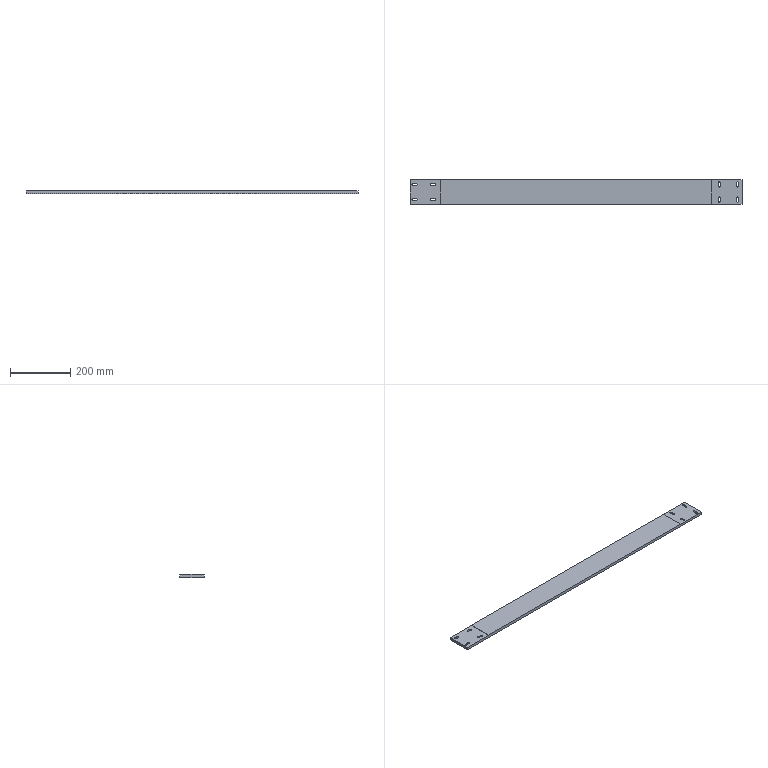Part | SolidWorks | features ICE 2, Extrusion 1, HoleWzd 1 | 1 solid | 46 faces | box 1100 x 80 x 10 mm | volume 856189 mm3 | plane 26 | cylinder 20 | commonest cylinder face diameters 7 x20
STEP:
#1=CARTESIAN_POINT('',(-540.,28.5,9.));
#2=VERTEX_POINT('',#1);
#3=CARTESIAN_POINT('',(-543.5,25.,9.));
#4=VERTEX_POINT('',#3);
#5=CARTESIAN_POINT('',(-540.,25.,9.));
#6=DIRECTION('',(0.,0.,1.));
#7=DIRECTION('',(1.,0.,0.));
#8=AXIS2_PLACEMENT_3D('',#5,#6,#7);
#9=CIRCLE('',#8,3.5);
#10=EDGE_CURVE('',#2,#4,#9,.T.);
#11=ORIENTED_EDGE('',*,*,#10,.T.);
#12=CARTESIAN_POINT('',(-543.5,25.,0.));
#13=VERTEX_POINT('',#12);
#14=CARTESIAN_POINT('',(-543.5,25.,10.));
#15=DIRECTION('',(0.,0.,-1.));
#16=VECTOR('',#15,1000.);
#17=LINE('',#14,#16);
#18=EDGE_CURVE('',#4,#13,#17,.T.);
#19=ORIENTED_EDGE('',*,*,#18,.T.);
#20=CARTESIAN_POINT('',(-540.,28.5,0.));
#21=VERTEX_POINT('',#20);
#22=CARTESIAN_POINT('',(-540.,25.,0.));
#23=DIRECTION('',(0.,0.,-1.));
#24=DIRECTION('',(-1.,0.,0.));
#25=AXIS2_PLACEMENT_3D('',#22,#23,#24);
#26=CIRCLE('',#25,3.5);
#27=EDGE_CURVE('',#13,#21,#26,.T.);
#28=ORIENTED_EDGE('',*,*,#27,.T.);
#29=CARTESIAN_POINT('',(-540.,28.5,10.));
#30=DIRECTION('',(0.,0.,-1.));
#31=VECTOR('',#30,1000.);
#32=LINE('',#29,#31);
#33=EDGE_CURVE('',#2,#21,#32,.T.);
#34=ORIENTED_EDGE('',*,*,#33,.F.);
#35=EDGE_LOOP('',(#11,#19,#28,#34));
#36=FACE_OUTER_BOUND('',#35,.T.);
#37=CARTESIAN_POINT('',(-540.,25.,10.));
#38=DIRECTION('',(0.,0.,-1.));
#39=DIRECTION('',(-1.,0.,0.));
#40=AXIS2_PLACEMENT_3D('',#37,#38,#39);
#41=CYLINDRICAL_SURFACE('',#40,3.5);
#42=ADVANCED_FACE('',(#36),#41,.F.);
#43=CARTESIAN_POINT('',(-540.,-21.5,9.));
#44=VERTEX_POINT('',#43);
#45=CARTESIAN_POINT('',(-543.5,-25.,9.));
#46=VERTEX_POINT('',#45);
#47=CARTESIAN_POINT('',(-540.,-25.,9.));
#48=DIRECTION('',(0.,0.,1.));
#49=DIRECTION('',(1.,0.,0.));
#50=AXIS2_PLACEMENT_3D('',#47,#48,#49);
#51=CIRCLE('',#50,3.5);
#52=EDGE_CURVE('',#44,#46,#51,.T.);
#53=ORIENTED_EDGE('',*,*,#52,.T.);
#54=CARTESIAN_POINT('',(-543.5,-25.,0.));
#55=VERTEX_POINT('',#54);
#56=CARTESIAN_POINT('',(-543.5,-25.,10.));
#57=DIRECTION('',(0.,0.,-1.));
#58=VECTOR('',#57,1000.);
#59=LINE('',#56,#58);
#60=EDGE_CURVE('',#46,#55,#59,.T.);
#61=ORIENTED_EDGE('',*,*,#60,.T.);
#62=CARTESIAN_POINT('',(-540.,-21.5,0.));
#63=VERTEX_POINT('',#62);
#64=CARTESIAN_POINT('',(-540.,-25.,0.));
#65=DIRECTION('',(0.,0.,-1.));
#66=DIRECTION('',(-1.,0.,0.));
#67=AXIS2_PLACEMENT_3D('',#64,#65,#66);
#68=CIRCLE('',#67,3.5);
#69=EDGE_CURVE('',#55,#63,#68,.T.);
#70=ORIENTED_EDGE('',*,*,#69,.T.);
#71=CARTESIAN_POINT('',(-540.,-21.5,10.));
#72=DIRECTION('',(0.,0.,-1.));
#73=VECTOR('',#72,1000.);
#74=LINE('',#71,#73);
#75=EDGE_CURVE('',#44,#63,#74,.T.);
#76=ORIENTED_EDGE('',*,*,#75,.F.);
#77=EDGE_LOOP('',(#53,#61,#70,#76));
#78=FACE_OUTER_BOUND('',#77,.T.);
#79=CARTESIAN_POINT('',(-540.,-25.,10.));
#80=DIRECTION('',(0.,0.,-1.));
#81=DIRECTION('',(-1.,0.,0.));
#82=AXIS2_PLACEMENT_3D('',#79,#80,#81);
#83=CYLINDRICAL_SURFACE('',#82,3.5);
#84=ADVANCED_FACE('',(#78),#83,.F.);
#85=CARTESIAN_POINT('',(-480.,-21.5,9.));
#86=VERTEX_POINT('',#85);
#87=CARTESIAN_POINT('',(-483.5,-25.,9.));
#88=VERTEX_POINT('',#87);
#89=CARTESIAN_POINT('',(-480.,-25.,9.));
#90=DIRECTION('',(0.,0.,1.));
#91=DIRECTION('',(1.,0.,0.));
#92=AXIS2_PLACEMENT_3D('',#89,#90,#91);
#93=CIRCLE('',#92,3.5);
#94=EDGE_CURVE('',#86,#88,#93,.T.);
#95=ORIENTED_EDGE('',*,*,#94,.T.);
#96=CARTESIAN_POINT('',(-483.5,-25.,0.));
#97=VERTEX_POINT('',#96);
#98=CARTESIAN_POINT('',(-483.5,-25.,10.));
#99=DIRECTION('',(0.,0.,-1.));
#100=VECTOR('',#99,1000.);
#101=LINE('',#98,#100);
#102=EDGE_CURVE('',#88,#97,#101,.T.);
#103=ORIENTED_EDGE('',*,*,#102,.T.);
#104=CARTESIAN_POINT('',(-480.,-21.5,0.));
#105=VERTEX_POINT('',#104);
#106=CARTESIAN_POINT('',(-480.,-25.,0.));
#107=DIRECTION('',(0.,0.,-1.));
#108=DIRECTION('',(-1.,0.,0.));
#109=AXIS2_PLACEMENT_3D('',#106,#107,#108);
#110=CIRCLE('',#109,3.5);
#111=EDGE_CURVE('',#97,#105,#110,.T.);
#112=ORIENTED_EDGE('',*,*,#111,.T.);
#113=CARTESIAN_POINT('',(-480.,-21.5,10.));
#114=DIRECTION('',(0.,0.,-1.));
#115=VECTOR('',#114,1000.);
#116=LINE('',#113,#115);
#117=EDGE_CURVE('',#86,#105,#116,.T.);
#118=ORIENTED_EDGE('',*,*,#117,.F.);
#119=EDGE_LOOP('',(#95,#103,#112,#118));
#120=FACE_OUTER_BOUND('',#119,.T.);
#121=CARTESIAN_POINT('',(-480.,-25.,10.));
#122=DIRECTION('',(0.,0.,-1.));
#123=DIRECTION('',(-1.,0.,0.));
#124=AXIS2_PLACEMENT_3D('',#121,#122,#123);
#125=CYLINDRICAL_SURFACE('',#124,3.5);
#126=ADVANCED_FACE('',(#120),#125,.F.);
#127=CARTESIAN_POINT('',(-480.,28.5,9.));
#128=VERTEX_POINT('',#127);
#129=CARTESIAN_POINT('',(-483.5,25.,9.));
#130=VERTEX_POINT('',#129);
#131=CARTESIAN_POINT('',(-480.,25.,9.));
#132=DIRECTION('',(0.,0.,1.));
#133=DIRECTION('',(1.,0.,0.));
#134=AXIS2_PLACEMENT_3D('',#131,#132,#133);
#135=CIRCLE('',#134,3.5);
#136=EDGE_CURVE('',#128,#130,#135,.T.);
#137=ORIENTED_EDGE('',*,*,#136,.T.);
#138=CARTESIAN_POINT('',(-483.5,25.,0.));
#139=VERTEX_POINT('',#138);
#140=CARTESIAN_POINT('',(-483.5,25.,10.));
#141=DIRECTION('',(0.,0.,-1.));
#142=VECTOR('',#141,1000.);
#143=LINE('',#140,#142);
#144=EDGE_CURVE('',#130,#139,#143,.T.);
#145=ORIENTED_EDGE('',*,*,#144,.T.);
#146=CARTESIAN_POINT('',(-480.,28.5,0.));
#147=VERTEX_POINT('',#146);
#148=CARTESIAN_POINT('',(-480.,25.,0.));
#149=DIRECTION('',(0.,0.,-1.));
#150=DIRECTION('',(-1.,0.,0.));
#151=AXIS2_PLACEMENT_3D('',#148,#149,#150);
#152=CIRCLE('',#151,3.5);
#153=EDGE_CURVE('',#139,#147,#152,.T.);
#154=ORIENTED_EDGE('',*,*,#153,.T.);
#155=CARTESIAN_POINT('',(-480.,28.5,10.));
#156=DIRECTION('',(0.,0.,-1.));
#157=VECTOR('',#156,1000.);
#158=LINE('',#155,#157);
#159=EDGE_CURVE('',#128,#147,#158,.T.);
#160=ORIENTED_EDGE('',*,*,#159,.F.);
#161=EDGE_LOOP('',(#137,#145,#154,#160));
#162=FACE_OUTER_BOUND('',#161,.T.);
#163=CARTESIAN_POINT('',(-480.,25.,10.));
#164=DIRECTION('',(0.,0.,-1.));
#165=DIRECTION('',(-1.,0.,0.));
#166=AXIS2_PLACEMENT_3D('',#163,#164,#165);
#167=CYLINDRICAL_SURFACE('',#166,3.5);
#168=ADVANCED_FACE('',(#162),#167,.F.);
#169=CARTESIAN_POINT('',(550.,-40.,9.));
#170=VERTEX_POINT('',#169);
#171=CARTESIAN_POINT('',(550.,40.,9.));
#172=VERTEX_POINT('',#171);
#173=CARTESIAN_POINT('',(550.,40.,9.));
#174=DIRECTION('',(0.,1.,0.));
#175=VECTOR('',#174,1000.);
#176=LINE('',#173,#175);
#177=EDGE_CURVE('',#170,#172,#176,.T.);
#178=ORIENTED_EDGE('',*,*,#177,.F.);
#179=CARTESIAN_POINT('',(550.,-40.,0.));
#180=VERTEX_POINT('',#179);
#181=CARTESIAN_POINT('',(550.,-40.,10.));
#182=DIRECTION('',(0.,0.,-1.));
#183=VECTOR('',#182,1000.);
#184=LINE('',#181,#183);
#185=EDGE_CURVE('',#170,#180,#184,.T.);
#186=ORIENTED_EDGE('',*,*,#185,.T.);
#187=CARTESIAN_POINT('',(550.,40.,0.));
#188=VERTEX_POINT('',#187);
#189=CARTESIAN_POINT('',(550.,40.,0.));
#190=DIRECTION('',(0.,1.,0.));
#191=VECTOR('',#190,1000.);
#192=LINE('',#189,#191);
#193=EDGE_CURVE('',#180,#188,#192,.T.);
#194=ORIENTED_EDGE('',*,*,#193,.T.);
#195=CARTESIAN_POINT('',(550.,40.,10.));
#196=DIRECTION('',(0.,0.,-1.));
#197=VECTOR('',#196,1000.);
#198=LINE('',#195,#197);
#199=EDGE_CURVE('',#172,#188,#198,.T.);
#200=ORIENTED_EDGE('',*,*,#199,.F.);
#201=EDGE_LOOP('',(#178,#186,#194,#200));
#202=FACE_OUTER_BOUND('',#201,.T.);
#203=CARTESIAN_POINT('',(550.,40.,10.));
#204=DIRECTION('',(-1.,0.,0.));
#205=DIRECTION('',(0.,0.,1.));
#206=AXIS2_PLACEMENT_3D('',#203,#204,#205);
#207=PLANE('',#206);
#208=ADVANCED_FACE('',(#202),#207,.F.);
#209=CARTESIAN_POINT('',(-550.,40.,9.));
#210=VERTEX_POINT('',#209);
#211=CARTESIAN_POINT('',(-550.,-40.,9.));
#212=VERTEX_POINT('',#211);
#213=CARTESIAN_POINT('',(-550.,40.,9.));
#214=DIRECTION('',(0.,-1.,0.));
#215=VECTOR('',#214,1000.);
#216=LINE('',#213,#215);
#217=EDGE_CURVE('',#210,#212,#216,.T.);
#218=ORIENTED_EDGE('',*,*,#217,.F.);
#219=CARTESIAN_POINT('',(-550.,40.,0.));
#220=VERTEX_POINT('',#219);
#221=CARTESIAN_POINT('',(-550.,40.,10.));
#222=DIRECTION('',(0.,0.,-1.));
#223=VECTOR('',#222,1000.);
#224=LINE('',#221,#223);
#225=EDGE_CURVE('',#210,#220,#224,.T.);
#226=ORIENTED_EDGE('',*,*,#225,.T.);
#227=CARTESIAN_POINT('',(-550.,-40.,0.));
#228=VERTEX_POINT('',#227);
#229=CARTESIAN_POINT('',(-550.,40.,0.));
#230=DIRECTION('',(0.,-1.,0.));
#231=VECTOR('',#230,1000.);
#232=LINE('',#229,#231);
#233=EDGE_CURVE('',#220,#228,#232,.T.);
#234=ORIENTED_EDGE('',*,*,#233,.T.);
#235=CARTESIAN_POINT('',(-550.,-40.,10.));
#236=DIRECTION('',(0.,0.,-1.));
#237=VECTOR('',#236,1000.);
#238=LINE('',#235,#237);
#239=EDGE_CURVE('',#212,#228,#238,.T.);
#240=ORIENTED_EDGE('',*,*,#239,.F.);
#241=EDGE_LOOP('',(#218,#226,#234,#240));
#242=FACE_OUTER_BOUND('',#241,.T.);
#243=CARTESIAN_POINT('',(-550.,40.,10.));
#244=DIRECTION('',(1.,0.,0.));
#245=DIRECTION('',(0.,0.,-1.));
#246=AXIS2_PLACEMENT_3D('',#243,#244,#245);
#247=PLANE('',#246);
#248=ADVANCED_FACE('',(#242),#247,.F.);
#249=CARTESIAN_POINT('',(-450.,40.,9.));
#250=VERTEX_POINT('',#249);
#251=CARTESIAN_POINT('',(-550.,40.,9.));
#252=DIRECTION('',(-1.,0.,0.));
#253=VECTOR('',#252,1000.);
#254=LINE('',#251,#253);
#255=EDGE_CURVE('',#250,#210,#254,.T.);
#256=ORIENTED_EDGE('',*,*,#255,.F.);
#257=CARTESIAN_POINT('',(-450.,40.,10.));
#258=VERTEX_POINT('',#257);
#259=CARTESIAN_POINT('',(-450.,40.,9.));
#260=DIRECTION('',(0.,0.,1.));
#261=VECTOR('',#260,1000.);
#262=LINE('',#259,#261);
#263=EDGE_CURVE('',#250,#258,#262,.T.);
#264=ORIENTED_EDGE('',*,*,#263,.T.);
#265=CARTESIAN_POINT('',(450.,40.,10.));
#266=VERTEX_POINT('',#265);
#267=CARTESIAN_POINT('',(-550.,40.,10.));
#268=DIRECTION('',(-1.,0.,0.));
#269=VECTOR('',#268,1000.);
#270=LINE('',#267,#269);
#271=EDGE_CURVE('',#266,#258,#270,.T.);
#272=ORIENTED_EDGE('',*,*,#271,.F.);
#273=CARTESIAN_POINT('',(450.,40.,9.));
#274=VERTEX_POINT('',#273);
#275=CARTESIAN_POINT('',(450.,40.,9.));
#276=DIRECTION('',(0.,0.,1.));
#277=VECTOR('',#276,1000.);
#278=LINE('',#275,#277);
#279=EDGE_CURVE('',#274,#266,#278,.T.);
#280=ORIENTED_EDGE('',*,*,#279,.F.);
#281=CARTESIAN_POINT('',(550.,40.,9.));
#282=DIRECTION('',(-1.,0.,0.));
#283=VECTOR('',#282,1000.);
#284=LINE('',#281,#283);
#285=EDGE_CURVE('',#172,#274,#284,.T.);
#286=ORIENTED_EDGE('',*,*,#285,.F.);
#287=ORIENTED_EDGE('',*,*,#199,.T.);
#288=CARTESIAN_POINT('',(-550.,40.,0.));
#289=DIRECTION('',(-1.,0.,0.));
#290=VECTOR('',#289,1000.);
#291=LINE('',#288,#290);
#292=EDGE_CURVE('',#188,#220,#291,.T.);
#293=ORIENTED_EDGE('',*,*,#292,.T.);
#294=ORIENTED_EDGE('',*,*,#225,.F.);
#295=EDGE_LOOP('',(#256,#264,#272,#280,#286,#287,#293,#294));
#296=FACE_OUTER_BOUND('',#295,.T.);
#297=CARTESIAN_POINT('',(-550.,40.,10.));
#298=DIRECTION('',(0.,-1.,0.));
#299=DIRECTION('',(0.,0.,-1.));
#300=AXIS2_PLACEMENT_3D('',#297,#298,#299);
#301=PLANE('',#300);
#302=ADVANCED_FACE('',(#296),#301,.F.);
#303=CARTESIAN_POINT('',(-450.,-40.,10.));
#304=VERTEX_POINT('',#303);
#305=CARTESIAN_POINT('',(450.,-40.,10.));
#306=VERTEX_POINT('',#305);
#307=CARTESIAN_POINT('',(-550.,-40.,10.));
#308=DIRECTION('',(1.,0.,0.));
#309=VECTOR('',#308,1000.);
#310=LINE('',#307,#309);
#311=EDGE_CURVE('',#304,#306,#310,.T.);
#312=ORIENTED_EDGE('',*,*,#311,.F.);
#313=CARTESIAN_POINT('',(-450.,-40.,9.));
#314=VERTEX_POINT('',#313);
#315=CARTESIAN_POINT('',(-450.,-40.,9.));
#316=DIRECTION('',(0.,0.,1.));
#317=VECTOR('',#316,1000.);
#318=LINE('',#315,#317);
#319=EDGE_CURVE('',#314,#304,#318,.T.);
#320=ORIENTED_EDGE('',*,*,#319,.F.);
#321=CARTESIAN_POINT('',(-550.,-40.,9.));
#322=DIRECTION('',(1.,0.,0.));
#323=VECTOR('',#322,1000.);
#324=LINE('',#321,#323);
#325=EDGE_CURVE('',#212,#314,#324,.T.);
#326=ORIENTED_EDGE('',*,*,#325,.F.);
#327=ORIENTED_EDGE('',*,*,#239,.T.);
#328=CARTESIAN_POINT('',(-550.,-40.,0.));
#329=DIRECTION('',(1.,0.,0.));
#330=VECTOR('',#329,1000.);
#331=LINE('',#328,#330);
#332=EDGE_CURVE('',#228,#180,#331,.T.);
#333=ORIENTED_EDGE('',*,*,#332,.T.);
#334=ORIENTED_EDGE('',*,*,#185,.F.);
#335=CARTESIAN_POINT('',(450.,-40.,9.));
#336=VERTEX_POINT('',#335);
#337=CARTESIAN_POINT('',(550.,-40.,9.));
#338=DIRECTION('',(1.,0.,0.));
#339=VECTOR('',#338,1000.);
#340=LINE('',#337,#339);
#341=EDGE_CURVE('',#336,#170,#340,.T.);
#342=ORIENTED_EDGE('',*,*,#341,.F.);
#343=CARTESIAN_POINT('',(450.,-40.,9.));
#344=DIRECTION('',(0.,0.,1.));
#345=VECTOR('',#344,1000.);
#346=LINE('',#343,#345);
#347=EDGE_CURVE('',#336,#306,#346,.T.);
#348=ORIENTED_EDGE('',*,*,#347,.T.);
#349=EDGE_LOOP('',(#312,#320,#326,#327,#333,#334,#342,#348));
#350=FACE_OUTER_BOUND('',#349,.T.);
#351=CARTESIAN_POINT('',(-550.,-40.,10.));
#352=DIRECTION('',(0.,1.,0.));
#353=DIRECTION('',(0.,0.,1.));
#354=AXIS2_PLACEMENT_3D('',#351,#352,#353);
#355=PLANE('',#354);
#356=ADVANCED_FACE('',(#350),#355,.F.);
#357=CARTESIAN_POINT('',(-450.,40.,10.));
#358=DIRECTION('',(0.,1.,0.));
#359=VECTOR('',#358,1000.);
#360=LINE('',#357,#359);
#361=EDGE_CURVE('',#304,#258,#360,.T.);
#362=ORIENTED_EDGE('',*,*,#361,.F.);
#363=ORIENTED_EDGE('',*,*,#311,.T.);
#364=CARTESIAN_POINT('',(450.,40.,10.));
#365=DIRECTION('',(0.,-1.,0.));
#366=VECTOR('',#365,1000.);
#367=LINE('',#364,#366);
#368=EDGE_CURVE('',#266,#306,#367,.T.);
#369=ORIENTED_EDGE('',*,*,#368,.F.);
#370=ORIENTED_EDGE('',*,*,#271,.T.);
#371=EDGE_LOOP('',(#362,#363,#369,#370));
#372=FACE_OUTER_BOUND('',#371,.T.);
#373=CARTESIAN_POINT('',(0.,0.,10.));
#374=DIRECTION('',(0.,0.,1.));
#375=DIRECTION('',(1.,0.,0.));
#376=AXIS2_PLACEMENT_3D('',#373,#374,#375);
#377=PLANE('',#376);
#378=ADVANCED_FACE('',(#372),#377,.T.);
#379=CARTESIAN_POINT('',(-470.,-28.5,0.));
#380=VERTEX_POINT('',#379);
#381=CARTESIAN_POINT('',(-480.,-28.5,0.));
#382=VERTEX_POINT('',#381);
#383=CARTESIAN_POINT('',(-470.,-28.5,0.));
#384=DIRECTION('',(-1.,0.,0.));
#385=VECTOR('',#384,1000.);
#386=LINE('',#383,#385);
#387=EDGE_CURVE('',#380,#382,#386,.T.);
#388=ORIENTED_EDGE('',*,*,#387,.F.);
#389=CARTESIAN_POINT('',(-470.,-21.5,0.));
#390=VERTEX_POINT('',#389);
#391=CARTESIAN_POINT('',(-470.,-25.,0.));
#392=DIRECTION('',(0.,0.,-1.));
#393=DIRECTION('',(-1.,0.,0.));
#394=AXIS2_PLACEMENT_3D('',#391,#392,#393);
#395=CIRCLE('',#394,3.5);
#396=EDGE_CURVE('',#390,#380,#395,.T.);
#397=ORIENTED_EDGE('',*,*,#396,.F.);
#398=CARTESIAN_POINT('',(-470.,-21.5,0.));
#399=DIRECTION('',(1.,0.,0.));
#400=VECTOR('',#399,1000.);
#401=LINE('',#398,#400);
#402=EDGE_CURVE('',#105,#390,#401,.T.);
#403=ORIENTED_EDGE('',*,*,#402,.F.);
#404=ORIENTED_EDGE('',*,*,#111,.F.);
#405=CARTESIAN_POINT('',(-480.,-25.,0.));
#406=DIRECTION('',(0.,0.,-1.));
#407=DIRECTION('',(-1.,0.,0.));
#408=AXIS2_PLACEMENT_3D('',#405,#406,#407);
#409=CIRCLE('',#408,3.5);
#410=EDGE_CURVE('',#382,#97,#409,.T.);
#411=ORIENTED_EDGE('',*,*,#410,.F.);
#412=EDGE_LOOP('',(#388,#397,#403,#404,#411));
#413=FACE_BOUND('',#412,.T.);
#414=CARTESIAN_POINT('',(-530.,21.5,0.));
#415=VERTEX_POINT('',#414);
#416=CARTESIAN_POINT('',(-540.,21.5,0.));
#417=VERTEX_POINT('',#416);
#418=CARTESIAN_POINT('',(-530.,21.5,0.));
#419=DIRECTION('',(-1.,0.,0.));
#420=VECTOR('',#419,1000.);
#421=LINE('',#418,#420);
#422=EDGE_CURVE('',#415,#417,#421,.T.);
#423=ORIENTED_EDGE('',*,*,#422,.F.);
#424=CARTESIAN_POINT('',(-530.,28.5,0.));
#425=VERTEX_POINT('',#424);
#426=CARTESIAN_POINT('',(-530.,25.,0.));
#427=DIRECTION('',(0.,0.,-1.));
#428=DIRECTION('',(-1.,0.,0.));
#429=AXIS2_PLACEMENT_3D('',#426,#427,#428);
#430=CIRCLE('',#429,3.5);
#431=EDGE_CURVE('',#425,#415,#430,.T.);
#432=ORIENTED_EDGE('',*,*,#431,.F.);
#433=CARTESIAN_POINT('',(-530.,28.5,0.));
#434=DIRECTION('',(1.,0.,0.));
#435=VECTOR('',#434,1000.);
#436=LINE('',#433,#435);
#437=EDGE_CURVE('',#21,#425,#436,.T.);
#438=ORIENTED_EDGE('',*,*,#437,.F.);
#439=ORIENTED_EDGE('',*,*,#27,.F.);
#440=CARTESIAN_POINT('',(-540.,25.,0.));
#441=DIRECTION('',(0.,0.,-1.));
#442=DIRECTION('',(-1.,0.,0.));
#443=AXIS2_PLACEMENT_3D('',#440,#441,#442);
#444=CIRCLE('',#443,3.5);
#445=EDGE_CURVE('',#417,#13,#444,.T.);
#446=ORIENTED_EDGE('',*,*,#445,.F.);
#447=EDGE_LOOP('',(#423,#432,#438,#439,#446));
#448=FACE_BOUND('',#447,.T.);
#449=CARTESIAN_POINT('',(-530.,-28.5,0.));
#450=VERTEX_POINT('',#449);
#451=CARTESIAN_POINT('',(-540.,-28.5,0.));
#452=VERTEX_POINT('',#451);
#453=CARTESIAN_POINT('',(-530.,-28.5,0.));
#454=DIRECTION('',(-1.,0.,0.));
#455=VECTOR('',#454,1000.);
#456=LINE('',#453,#455);
#457=EDGE_CURVE('',#450,#452,#456,.T.);
#458=ORIENTED_EDGE('',*,*,#457,.F.);
#459=CARTESIAN_POINT('',(-530.,-21.5,0.));
#460=VERTEX_POINT('',#459);
#461=CARTESIAN_POINT('',(-530.,-25.,0.));
#462=DIRECTION('',(0.,0.,-1.));
#463=DIRECTION('',(-1.,0.,0.));
#464=AXIS2_PLACEMENT_3D('',#461,#462,#463);
#465=CIRCLE('',#464,3.5);
#466=EDGE_CURVE('',#460,#450,#465,.T.);
#467=ORIENTED_EDGE('',*,*,#466,.F.);
#468=CARTESIAN_POINT('',(-530.,-21.5,0.));
#469=DIRECTION('',(1.,0.,0.));
#470=VECTOR('',#469,1000.);
#471=LINE('',#468,#470);
#472=EDGE_CURVE('',#63,#460,#471,.T.);
#473=ORIENTED_EDGE('',*,*,#472,.F.);
#474=ORIENTED_EDGE('',*,*,#69,.F.);
#475=CARTESIAN_POINT('',(-540.,-25.,0.));
#476=DIRECTION('',(0.,0.,-1.));
#477=DIRECTION('',(-1.,0.,0.));
#478=AXIS2_PLACEMENT_3D('',#475,#476,#477);
#479=CIRCLE('',#478,3.5);
#480=EDGE_CURVE('',#452,#55,#479,.T.);
#481=ORIENTED_EDGE('',*,*,#480,.F.);
#482=EDGE_LOOP('',(#458,#467,#473,#474,#481));
#483=FACE_BOUND('',#482,.T.);
#484=CARTESIAN_POINT('',(-470.,21.5,0.));
#485=VERTEX_POINT('',#484);
#486=CARTESIAN_POINT('',(-480.,21.5,0.));
#487=VERTEX_POINT('',#486);
#488=CARTESIAN_POINT('',(-470.,21.5,0.));
#489=DIRECTION('',(-1.,0.,0.));
#490=VECTOR('',#489,1000.);
#491=LINE('',#488,#490);
#492=EDGE_CURVE('',#485,#487,#491,.T.);
#493=ORIENTED_EDGE('',*,*,#492,.F.);
#494=CARTESIAN_POINT('',(-470.,28.5,0.));
#495=VERTEX_POINT('',#494);
#496=CARTESIAN_POINT('',(-470.,25.,0.));
#497=DIRECTION('',(0.,0.,-1.));
#498=DIRECTION('',(-1.,0.,0.));
#499=AXIS2_PLACEMENT_3D('',#496,#497,#498);
#500=CIRCLE('',#499,3.5);
#501=EDGE_CURVE('',#495,#485,#500,.T.);
#502=ORIENTED_EDGE('',*,*,#501,.F.);
#503=CARTESIAN_POINT('',(-470.,28.5,0.));
#504=DIRECTION('',(1.,0.,0.));
#505=VECTOR('',#504,1000.);
#506=LINE('',#503,#505);
#507=EDGE_CURVE('',#147,#495,#506,.T.);
#508=ORIENTED_EDGE('',*,*,#507,.F.);
#509=ORIENTED_EDGE('',*,*,#153,.F.);
#510=CARTESIAN_POINT('',(-480.,25.,0.));
#511=DIRECTION('',(0.,0.,-1.));
#512=DIRECTION('',(-1.,0.,0.));
#513=AXIS2_PLACEMENT_3D('',#510,#511,#512);
#514=CIRCLE('',#513,3.5);
#515=EDGE_CURVE('',#487,#139,#514,.T.);
#516=ORIENTED_EDGE('',*,*,#515,.F.);
#517=EDGE_LOOP('',(#493,#502,#508,#509,#516));
#518=FACE_BOUND('',#517,.T.);
#519=CARTESIAN_POINT('',(478.5,30.,0.));
#520=VERTEX_POINT('',#519);
#521=CARTESIAN_POINT('',(478.5,20.,0.));
#522=VERTEX_POINT('',#521);
#523=CARTESIAN_POINT('',(478.5,30.,0.));
#524=DIRECTION('',(0.,-1.,0.));
#525=VECTOR('',#524,1000.);
#526=LINE('',#523,#525);
#527=EDGE_CURVE('',#520,#522,#526,.T.);
#528=ORIENTED_EDGE('',*,*,#527,.F.);
#529=CARTESIAN_POINT('',(471.5,30.,0.));
#530=VERTEX_POINT('',#529);
#531=CARTESIAN_POINT('',(475.,30.,0.));
#532=DIRECTION('',(0.,0.,-1.));
#533=DIRECTION('',(-1.,0.,0.));
#534=AXIS2_PLACEMENT_3D('',#531,#532,#533);
#535=CIRCLE('',#534,3.5);
#536=EDGE_CURVE('',#530,#520,#535,.T.);
#537=ORIENTED_EDGE('',*,*,#536,.F.);
#538=CARTESIAN_POINT('',(471.5,20.,0.));
#539=VERTEX_POINT('',#538);
#540=CARTESIAN_POINT('',(471.5,30.,0.));
#541=DIRECTION('',(0.,1.,0.));
#542=VECTOR('',#541,1000.);
#543=LINE('',#540,#542);
#544=EDGE_CURVE('',#539,#530,#543,.T.);
#545=ORIENTED_EDGE('',*,*,#544,.F.);
#546=CARTESIAN_POINT('',(475.,20.,0.));
#547=DIRECTION('',(0.,0.,-1.));
#548=DIRECTION('',(-1.,0.,0.));
#549=AXIS2_PLACEMENT_3D('',#546,#547,#548);
#550=CIRCLE('',#549,3.5);
#551=EDGE_CURVE('',#522,#539,#550,.T.);
#552=ORIENTED_EDGE('',*,*,#551,.F.);
#553=EDGE_LOOP('',(#528,#537,#545,#552));
#554=FACE_BOUND('',#553,.T.);
#555=CARTESIAN_POINT('',(471.5,-30.,0.));
#556=VERTEX_POINT('',#555);
#557=CARTESIAN_POINT('',(471.5,-20.,0.));
#558=VERTEX_POINT('',#557);
#559=CARTESIAN_POINT('',(471.5,-30.,0.));
#560=DIRECTION('',(0.,1.,0.));
#561=VECTOR('',#560,1000.);
#562=LINE('',#559,#561);
#563=EDGE_CURVE('',#556,#558,#562,.T.);
#564=ORIENTED_EDGE('',*,*,#563,.F.);
#565=CARTESIAN_POINT('',(478.5,-30.,0.));
#566=VERTEX_POINT('',#565);
#567=CARTESIAN_POINT('',(475.,-30.,0.));
#568=DIRECTION('',(0.,0.,-1.));
#569=DIRECTION('',(-1.,0.,0.));
#570=AXIS2_PLACEMENT_3D('',#567,#568,#569);
#571=CIRCLE('',#570,3.5);
#572=EDGE_CURVE('',#566,#556,#571,.T.);
#573=ORIENTED_EDGE('',*,*,#572,.F.);
#574=CARTESIAN_POINT('',(478.5,-20.,0.));
#575=VERTEX_POINT('',#574);
#576=CARTESIAN_POINT('',(478.5,-30.,0.));
#577=DIRECTION('',(0.,-1.,0.));
#578=VECTOR('',#577,1000.);
#579=LINE('',#576,#578);
#580=EDGE_CURVE('',#575,#566,#579,.T.);
#581=ORIENTED_EDGE('',*,*,#580,.F.);
#582=CARTESIAN_POINT('',(475.,-20.,0.));
#583=DIRECTION('',(0.,0.,-1.));
#584=DIRECTION('',(-1.,0.,0.));
#585=AXIS2_PLACEMENT_3D('',#582,#583,#584);
#586=CIRCLE('',#585,3.5);
#587=EDGE_CURVE('',#558,#575,#586,.T.);
#588=ORIENTED_EDGE('',*,*,#587,.F.);
#589=EDGE_LOOP('',(#564,#573,#581,#588));
#590=FACE_BOUND('',#589,.T.);
#591=CARTESIAN_POINT('',(531.5,-30.,0.));
#592=VERTEX_POINT('',#591);
#593=CARTESIAN_POINT('',(531.5,-20.,0.));
#594=VERTEX_POINT('',#593);
#595=CARTESIAN_POINT('',(531.5,-30.,0.));
#596=DIRECTION('',(0.,1.,0.));
#597=VECTOR('',#596,1000.);
#598=LINE('',#595,#597);
#599=EDGE_CURVE('',#592,#594,#598,.T.);
#600=ORIENTED_EDGE('',*,*,#599,.F.);
#601=CARTESIAN_POINT('',(538.5,-30.,0.));
#602=VERTEX_POINT('',#601);
#603=CARTESIAN_POINT('',(535.,-30.,0.));
#604=DIRECTION('',(0.,0.,-1.));
#605=DIRECTION('',(-1.,0.,0.));
#606=AXIS2_PLACEMENT_3D('',#603,#604,#605);
#607=CIRCLE('',#606,3.5);
#608=EDGE_CURVE('',#602,#592,#607,.T.);
#609=ORIENTED_EDGE('',*,*,#608,.F.);
#610=CARTESIAN_POINT('',(538.5,-20.,0.));
#611=VERTEX_POINT('',#610);
#612=CARTESIAN_POINT('',(538.5,-30.,0.));
#613=DIRECTION('',(0.,-1.,0.));
#614=VECTOR('',#613,1000.);
#615=LINE('',#612,#614);
#616=EDGE_CURVE('',#611,#602,#615,.T.);
#617=ORIENTED_EDGE('',*,*,#616,.F.);
#618=CARTESIAN_POINT('',(535.,-20.,0.));
#619=DIRECTION('',(0.,0.,-1.));
#620=DIRECTION('',(-1.,0.,0.));
#621=AXIS2_PLACEMENT_3D('',#618,#619,#620);
#622=CIRCLE('',#621,3.5);
#623=EDGE_CURVE('',#594,#611,#622,.T.);
#624=ORIENTED_EDGE('',*,*,#623,.F.);
#625=EDGE_LOOP('',(#600,#609,#617,#624));
#626=FACE_BOUND('',#625,.T.);
#627=CARTESIAN_POINT('',(538.5,30.,0.));
#628=VERTEX_POINT('',#627);
#629=CARTESIAN_POINT('',(538.5,20.,0.));
#630=VERTEX_POINT('',#629);
#631=CARTESIAN_POINT('',(538.5,30.,0.));
#632=DIRECTION('',(0.,-1.,0.));
#633=VECTOR('',#632,1000.);
#634=LINE('',#631,#633);
#635=EDGE_CURVE('',#628,#630,#634,.T.);
#636=ORIENTED_EDGE('',*,*,#635,.F.);
#637=CARTESIAN_POINT('',(531.5,30.,0.));
#638=VERTEX_POINT('',#637);
#639=CARTESIAN_POINT('',(535.,30.,0.));
#640=DIRECTION('',(0.,0.,-1.));
#641=DIRECTION('',(-1.,0.,0.));
#642=AXIS2_PLACEMENT_3D('',#639,#640,#641);
#643=CIRCLE('',#642,3.5);
#644=EDGE_CURVE('',#638,#628,#643,.T.);
#645=ORIENTED_EDGE('',*,*,#644,.F.);
#646=CARTESIAN_POINT('',(531.5,20.,0.));
#647=VERTEX_POINT('',#646);
#648=CARTESIAN_POINT('',(531.5,30.,0.));
#649=DIRECTION('',(0.,1.,0.));
#650=VECTOR('',#649,1000.);
#651=LINE('',#648,#650);
#652=EDGE_CURVE('',#647,#638,#651,.T.);
#653=ORIENTED_EDGE('',*,*,#652,.F.);
#654=CARTESIAN_POINT('',(535.,20.,0.));
#655=DIRECTION('',(0.,0.,-1.));
#656=DIRECTION('',(-1.,0.,0.));
#657=AXIS2_PLACEMENT_3D('',#654,#655,#656);
#658=CIRCLE('',#657,3.5);
#659=EDGE_CURVE('',#630,#647,#658,.T.);
#660=ORIENTED_EDGE('',*,*,#659,.F.);
#661=EDGE_LOOP('',(#636,#645,#653,#660));
#662=FACE_BOUND('',#661,.T.);
#663=ORIENTED_EDGE('',*,*,#193,.F.);
#664=ORIENTED_EDGE('',*,*,#332,.F.);
#665=ORIENTED_EDGE('',*,*,#233,.F.);
#666=ORIENTED_EDGE('',*,*,#292,.F.);
#667=EDGE_LOOP('',(#663,#664,#665,#666));
#668=FACE_OUTER_BOUND('',#667,.T.);
#669=CARTESIAN_POINT('',(0.,0.,0.));
#670=DIRECTION('',(0.,0.,1.));
#671=DIRECTION('',(1.,0.,0.));
#672=AXIS2_PLACEMENT_3D('',#669,#670,#671);
#673=PLANE('',#672);
#674=ADVANCED_FACE('',(#413,#448,#483,#518,#554,#590,#626,#662,#668),#673,.F.);
#675=ORIENTED_EDGE('',*,*,#368,.T.);
#676=ORIENTED_EDGE('',*,*,#347,.F.);
#677=CARTESIAN_POINT('',(450.,40.,9.));
#678=DIRECTION('',(0.,-1.,0.));
#679=VECTOR('',#678,1000.);
#680=LINE('',#677,#679);
#681=EDGE_CURVE('',#274,#336,#680,.T.);
#682=ORIENTED_EDGE('',*,*,#681,.F.);
#683=ORIENTED_EDGE('',*,*,#279,.T.);
#684=EDGE_LOOP('',(#675,#676,#682,#683));
#685=FACE_OUTER_BOUND('',#684,.T.);
#686=CARTESIAN_POINT('',(450.,40.,9.));
#687=DIRECTION('',(-1.,0.,0.));
#688=DIRECTION('',(0.,0.,1.));
#689=AXIS2_PLACEMENT_3D('',#686,#687,#688);
#690=PLANE('',#689);
#691=ADVANCED_FACE('',(#685),#690,.F.);
#692=CARTESIAN_POINT('',(538.5,30.,9.));
#693=VERTEX_POINT('',#692);
#694=CARTESIAN_POINT('',(531.5,30.,9.));
#695=VERTEX_POINT('',#694);
#696=CARTESIAN_POINT('',(535.,30.,9.));
#697=DIRECTION('',(0.,0.,1.));
#698=DIRECTION('',(1.,0.,0.));
#699=AXIS2_PLACEMENT_3D('',#696,#697,#698);
#700=CIRCLE('',#699,3.5);
#701=EDGE_CURVE('',#693,#695,#700,.T.);
#702=ORIENTED_EDGE('',*,*,#701,.F.);
#703=CARTESIAN_POINT('',(538.5,20.,9.));
#704=VERTEX_POINT('',#703);
#705=CARTESIAN_POINT('',(538.5,0.,9.));
#706=DIRECTION('',(0.,1.,0.));
#707=VECTOR('',#706,1000.);
#708=LINE('',#705,#707);
#709=EDGE_CURVE('',#704,#693,#708,.T.);
#710=ORIENTED_EDGE('',*,*,#709,.F.);
#711=CARTESIAN_POINT('',(531.5,20.,9.));
#712=VERTEX_POINT('',#711);
#713=CARTESIAN_POINT('',(535.,20.,9.));
#714=DIRECTION('',(0.,0.,1.));
#715=DIRECTION('',(1.,0.,0.));
#716=AXIS2_PLACEMENT_3D('',#713,#714,#715);
#717=CIRCLE('',#716,3.5);
#718=EDGE_CURVE('',#712,#704,#717,.T.);
#719=ORIENTED_EDGE('',*,*,#718,.F.);
#720=CARTESIAN_POINT('',(531.5,0.,9.));
#721=DIRECTION('',(0.,-1.,0.));
#722=VECTOR('',#721,1000.);
#723=LINE('',#720,#722);
#724=EDGE_CURVE('',#695,#712,#723,.T.);
#725=ORIENTED_EDGE('',*,*,#724,.F.);
#726=EDGE_LOOP('',(#702,#710,#719,#725));
#727=FACE_BOUND('',#726,.T.);
#728=CARTESIAN_POINT('',(471.5,-30.,9.));
#729=VERTEX_POINT('',#728);
#730=CARTESIAN_POINT('',(478.5,-30.,9.));
#731=VERTEX_POINT('',#730);
#732=CARTESIAN_POINT('',(475.,-30.,9.));
#733=DIRECTION('',(0.,0.,1.));
#734=DIRECTION('',(1.,0.,0.));
#735=AXIS2_PLACEMENT_3D('',#732,#733,#734);
#736=CIRCLE('',#735,3.5);
#737=EDGE_CURVE('',#729,#731,#736,.T.);
#738=ORIENTED_EDGE('',*,*,#737,.F.);
#739=CARTESIAN_POINT('',(471.5,-20.,9.));
#740=VERTEX_POINT('',#739);
#741=CARTESIAN_POINT('',(471.5,0.,9.));
#742=DIRECTION('',(0.,-1.,0.));
#743=VECTOR('',#742,1000.);
#744=LINE('',#741,#743);
#745=EDGE_CURVE('',#740,#729,#744,.T.);
#746=ORIENTED_EDGE('',*,*,#745,.F.);
#747=CARTESIAN_POINT('',(478.5,-20.,9.));
#748=VERTEX_POINT('',#747);
#749=CARTESIAN_POINT('',(475.,-20.,9.));
#750=DIRECTION('',(0.,0.,1.));
#751=DIRECTION('',(1.,0.,0.));
#752=AXIS2_PLACEMENT_3D('',#749,#750,#751);
#753=CIRCLE('',#752,3.5);
#754=EDGE_CURVE('',#748,#740,#753,.T.);
#755=ORIENTED_EDGE('',*,*,#754,.F.);
#756=CARTESIAN_POINT('',(478.5,0.,9.));
#757=DIRECTION('',(0.,1.,0.));
#758=VECTOR('',#757,1000.);
#759=LINE('',#756,#758);
#760=EDGE_CURVE('',#731,#748,#759,.T.);
#761=ORIENTED_EDGE('',*,*,#760,.F.);
#762=EDGE_LOOP('',(#738,#746,#755,#761));
#763=FACE_BOUND('',#762,.T.);
#764=CARTESIAN_POINT('',(531.5,-30.,9.));
#765=VERTEX_POINT('',#764);
#766=CARTESIAN_POINT('',(538.5,-30.,9.));
#767=VERTEX_POINT('',#766);
#768=CARTESIAN_POINT('',(535.,-30.,9.));
#769=DIRECTION('',(0.,0.,1.));
#770=DIRECTION('',(1.,0.,0.));
#771=AXIS2_PLACEMENT_3D('',#768,#769,#770);
#772=CIRCLE('',#771,3.5);
#773=EDGE_CURVE('',#765,#767,#772,.T.);
#774=ORIENTED_EDGE('',*,*,#773,.F.);
#775=CARTESIAN_POINT('',(531.5,-20.,9.));
#776=VERTEX_POINT('',#775);
#777=CARTESIAN_POINT('',(531.5,0.,9.));
#778=DIRECTION('',(0.,-1.,0.));
#779=VECTOR('',#778,1000.);
#780=LINE('',#777,#779);
#781=EDGE_CURVE('',#776,#765,#780,.T.);
#782=ORIENTED_EDGE('',*,*,#781,.F.);
#783=CARTESIAN_POINT('',(538.5,-20.,9.));
#784=VERTEX_POINT('',#783);
#785=CARTESIAN_POINT('',(535.,-20.,9.));
#786=DIRECTION('',(0.,0.,1.));
#787=DIRECTION('',(1.,0.,0.));
#788=AXIS2_PLACEMENT_3D('',#785,#786,#787);
#789=CIRCLE('',#788,3.5);
#790=EDGE_CURVE('',#784,#776,#789,.T.);
#791=ORIENTED_EDGE('',*,*,#790,.F.);
#792=CARTESIAN_POINT('',(538.5,0.,9.));
#793=DIRECTION('',(0.,1.,0.));
#794=VECTOR('',#793,1000.);
#795=LINE('',#792,#794);
#796=EDGE_CURVE('',#767,#784,#795,.T.);
#797=ORIENTED_EDGE('',*,*,#796,.F.);
#798=EDGE_LOOP('',(#774,#782,#791,#797));
#799=FACE_BOUND('',#798,.T.);
#800=CARTESIAN_POINT('',(478.5,30.,9.));
#801=VERTEX_POINT('',#800);
#802=CARTESIAN_POINT('',(471.5,30.,9.));
#803=VERTEX_POINT('',#802);
#804=CARTESIAN_POINT('',(475.,30.,9.));
#805=DIRECTION('',(0.,0.,1.));
#806=DIRECTION('',(1.,0.,0.));
#807=AXIS2_PLACEMENT_3D('',#804,#805,#806);
#808=CIRCLE('',#807,3.5);
#809=EDGE_CURVE('',#801,#803,#808,.T.);
#810=ORIENTED_EDGE('',*,*,#809,.F.);
#811=CARTESIAN_POINT('',(478.5,20.,9.));
#812=VERTEX_POINT('',#811);
#813=CARTESIAN_POINT('',(478.5,0.,9.));
#814=DIRECTION('',(0.,1.,0.));
#815=VECTOR('',#814,1000.);
#816=LINE('',#813,#815);
#817=EDGE_CURVE('',#812,#801,#816,.T.);
#818=ORIENTED_EDGE('',*,*,#817,.F.);
#819=CARTESIAN_POINT('',(471.5,20.,9.));
#820=VERTEX_POINT('',#819);
#821=CARTESIAN_POINT('',(475.,20.,9.));
#822=DIRECTION('',(0.,0.,1.));
#823=DIRECTION('',(1.,0.,0.));
#824=AXIS2_PLACEMENT_3D('',#821,#822,#823);
#825=CIRCLE('',#824,3.5);
#826=EDGE_CURVE('',#820,#812,#825,.T.);
#827=ORIENTED_EDGE('',*,*,#826,.F.);
#828=CARTESIAN_POINT('',(471.5,0.,9.));
#829=DIRECTION('',(0.,-1.,0.));
#830=VECTOR('',#829,1000.);
#831=LINE('',#828,#830);
#832=EDGE_CURVE('',#803,#820,#831,.T.);
#833=ORIENTED_EDGE('',*,*,#832,.F.);
#834=EDGE_LOOP('',(#810,#818,#827,#833));
#835=FACE_BOUND('',#834,.T.);
#836=ORIENTED_EDGE('',*,*,#285,.T.);
#837=ORIENTED_EDGE('',*,*,#681,.T.);
#838=ORIENTED_EDGE('',*,*,#341,.T.);
#839=ORIENTED_EDGE('',*,*,#177,.T.);
#840=EDGE_LOOP('',(#836,#837,#838,#839));
#841=FACE_OUTER_BOUND('',#840,.T.);
#842=CARTESIAN_POINT('',(0.,0.,9.));
#843=DIRECTION('',(0.,0.,1.));
#844=DIRECTION('',(1.,0.,0.));
#845=AXIS2_PLACEMENT_3D('',#842,#843,#844);
#846=PLANE('',#845);
#847=ADVANCED_FACE('',(#727,#763,#799,#835,#841),#846,.T.);
#848=ORIENTED_EDGE('',*,*,#361,.T.);
#849=ORIENTED_EDGE('',*,*,#263,.F.);
#850=CARTESIAN_POINT('',(-450.,40.,9.));
#851=DIRECTION('',(0.,1.,0.));
#852=VECTOR('',#851,1000.);
#853=LINE('',#850,#852);
#854=EDGE_CURVE('',#314,#250,#853,.T.);
#855=ORIENTED_EDGE('',*,*,#854,.F.);
#856=ORIENTED_EDGE('',*,*,#319,.T.);
#857=EDGE_LOOP('',(#848,#849,#855,#856));
#858=FACE_OUTER_BOUND('',#857,.T.);
#859=CARTESIAN_POINT('',(-450.,40.,9.));
#860=DIRECTION('',(1.,0.,0.));
#861=DIRECTION('',(0.,0.,-1.));
#862=AXIS2_PLACEMENT_3D('',#859,#860,#861);
#863=PLANE('',#862);
#864=ADVANCED_FACE('',(#858),#863,.F.);
#865=CARTESIAN_POINT('',(-530.,21.5,9.));
#866=VERTEX_POINT('',#865);
#867=CARTESIAN_POINT('',(-530.,28.5,9.));
#868=VERTEX_POINT('',#867);
#869=CARTESIAN_POINT('',(-530.,25.,9.));
#870=DIRECTION('',(0.,0.,1.));
#871=DIRECTION('',(1.,0.,0.));
#872=AXIS2_PLACEMENT_3D('',#869,#870,#871);
#873=CIRCLE('',#872,3.5);
#874=EDGE_CURVE('',#866,#868,#873,.T.);
#875=ORIENTED_EDGE('',*,*,#874,.F.);
#876=CARTESIAN_POINT('',(-540.,21.5,9.));
#877=VERTEX_POINT('',#876);
#878=CARTESIAN_POINT('',(0.,21.5,9.));
#879=DIRECTION('',(1.,0.,0.));
#880=VECTOR('',#879,1000.);
#881=LINE('',#878,#880);
#882=EDGE_CURVE('',#877,#866,#881,.T.);
#883=ORIENTED_EDGE('',*,*,#882,.F.);
#884=CARTESIAN_POINT('',(-540.,25.,9.));
#885=DIRECTION('',(0.,0.,1.));
#886=DIRECTION('',(1.,0.,0.));
#887=AXIS2_PLACEMENT_3D('',#884,#885,#886);
#888=CIRCLE('',#887,3.5);
#889=EDGE_CURVE('',#4,#877,#888,.T.);
#890=ORIENTED_EDGE('',*,*,#889,.F.);
#891=ORIENTED_EDGE('',*,*,#10,.F.);
#892=CARTESIAN_POINT('',(0.,28.5,9.));
#893=DIRECTION('',(-1.,0.,0.));
#894=VECTOR('',#893,1000.);
#895=LINE('',#892,#894);
#896=EDGE_CURVE('',#868,#2,#895,.T.);
#897=ORIENTED_EDGE('',*,*,#896,.F.);
#898=EDGE_LOOP('',(#875,#883,#890,#891,#897));
#899=FACE_BOUND('',#898,.T.);
#900=CARTESIAN_POINT('',(-530.,-28.5,9.));
#901=VERTEX_POINT('',#900);
#902=CARTESIAN_POINT('',(-530.,-21.5,9.));
#903=VERTEX_POINT('',#902);
#904=CARTESIAN_POINT('',(-530.,-25.,9.));
#905=DIRECTION('',(0.,0.,1.));
#906=DIRECTION('',(1.,0.,0.));
#907=AXIS2_PLACEMENT_3D('',#904,#905,#906);
#908=CIRCLE('',#907,3.5);
#909=EDGE_CURVE('',#901,#903,#908,.T.);
#910=ORIENTED_EDGE('',*,*,#909,.F.);
#911=CARTESIAN_POINT('',(-540.,-28.5,9.));
#912=VERTEX_POINT('',#911);
#913=CARTESIAN_POINT('',(0.,-28.5,9.));
#914=DIRECTION('',(1.,0.,0.));
#915=VECTOR('',#914,1000.);
#916=LINE('',#913,#915);
#917=EDGE_CURVE('',#912,#901,#916,.T.);
#918=ORIENTED_EDGE('',*,*,#917,.F.);
#919=CARTESIAN_POINT('',(-540.,-25.,9.));
#920=DIRECTION('',(0.,0.,1.));
#921=DIRECTION('',(1.,0.,0.));
#922=AXIS2_PLACEMENT_3D('',#919,#920,#921);
#923=CIRCLE('',#922,3.5);
#924=EDGE_CURVE('',#46,#912,#923,.T.);
#925=ORIENTED_EDGE('',*,*,#924,.F.);
#926=ORIENTED_EDGE('',*,*,#52,.F.);
#927=CARTESIAN_POINT('',(0.,-21.5,9.));
#928=DIRECTION('',(-1.,0.,0.));
#929=VECTOR('',#928,1000.);
#930=LINE('',#927,#929);
#931=EDGE_CURVE('',#903,#44,#930,.T.);
#932=ORIENTED_EDGE('',*,*,#931,.F.);
#933=EDGE_LOOP('',(#910,#918,#925,#926,#932));
#934=FACE_BOUND('',#933,.T.);
#935=CARTESIAN_POINT('',(-470.,-28.5,9.));
#936=VERTEX_POINT('',#935);
#937=CARTESIAN_POINT('',(-470.,-21.5,9.));
#938=VERTEX_POINT('',#937);
#939=CARTESIAN_POINT('',(-470.,-25.,9.));
#940=DIRECTION('',(0.,0.,1.));
#941=DIRECTION('',(1.,0.,0.));
#942=AXIS2_PLACEMENT_3D('',#939,#940,#941);
#943=CIRCLE('',#942,3.5);
#944=EDGE_CURVE('',#936,#938,#943,.T.);
#945=ORIENTED_EDGE('',*,*,#944,.F.);
#946=CARTESIAN_POINT('',(-480.,-28.5,9.));
#947=VERTEX_POINT('',#946);
#948=CARTESIAN_POINT('',(0.,-28.5,9.));
#949=DIRECTION('',(1.,0.,0.));
#950=VECTOR('',#949,1000.);
#951=LINE('',#948,#950);
#952=EDGE_CURVE('',#947,#936,#951,.T.);
#953=ORIENTED_EDGE('',*,*,#952,.F.);
#954=CARTESIAN_POINT('',(-480.,-25.,9.));
#955=DIRECTION('',(0.,0.,1.));
#956=DIRECTION('',(1.,0.,0.));
#957=AXIS2_PLACEMENT_3D('',#954,#955,#956);
#958=CIRCLE('',#957,3.5);
#959=EDGE_CURVE('',#88,#947,#958,.T.);
#960=ORIENTED_EDGE('',*,*,#959,.F.);
#961=ORIENTED_EDGE('',*,*,#94,.F.);
#962=CARTESIAN_POINT('',(0.,-21.5,9.));
#963=DIRECTION('',(-1.,0.,0.));
#964=VECTOR('',#963,1000.);
#965=LINE('',#962,#964);
#966=EDGE_CURVE('',#938,#86,#965,.T.);
#967=ORIENTED_EDGE('',*,*,#966,.F.);
#968=EDGE_LOOP('',(#945,#953,#960,#961,#967));
#969=FACE_BOUND('',#968,.T.);
#970=CARTESIAN_POINT('',(-470.,21.5,9.));
#971=VERTEX_POINT('',#970);
#972=CARTESIAN_POINT('',(-470.,28.5,9.));
#973=VERTEX_POINT('',#972);
#974=CARTESIAN_POINT('',(-470.,25.,9.));
#975=DIRECTION('',(0.,0.,1.));
#976=DIRECTION('',(1.,0.,0.));
#977=AXIS2_PLACEMENT_3D('',#974,#975,#976);
#978=CIRCLE('',#977,3.5);
#979=EDGE_CURVE('',#971,#973,#978,.T.);
#980=ORIENTED_EDGE('',*,*,#979,.F.);
#981=CARTESIAN_POINT('',(-480.,21.5,9.));
#982=VERTEX_POINT('',#981);
#983=CARTESIAN_POINT('',(0.,21.5,9.));
#984=DIRECTION('',(1.,0.,0.));
#985=VECTOR('',#984,1000.);
#986=LINE('',#983,#985);
#987=EDGE_CURVE('',#982,#971,#986,.T.);
#988=ORIENTED_EDGE('',*,*,#987,.F.);
#989=CARTESIAN_POINT('',(-480.,25.,9.));
#990=DIRECTION('',(0.,0.,1.));
#991=DIRECTION('',(1.,0.,0.));
#992=AXIS2_PLACEMENT_3D('',#989,#990,#991);
#993=CIRCLE('',#992,3.5);
#994=EDGE_CURVE('',#130,#982,#993,.T.);
#995=ORIENTED_EDGE('',*,*,#994,.F.);
#996=ORIENTED_EDGE('',*,*,#136,.F.);
#997=CARTESIAN_POINT('',(0.,28.5,9.));
#998=DIRECTION('',(-1.,0.,0.));
#999=VECTOR('',#998,1000.);
#1000=LINE('',#997,#999);
#1001=EDGE_CURVE('',#973,#128,#1000,.T.);
#1002=ORIENTED_EDGE('',*,*,#1001,.F.);
#1003=EDGE_LOOP('',(#980,#988,#995,#996,#1002));
#1004=FACE_BOUND('',#1003,.T.);
#1005=ORIENTED_EDGE('',*,*,#217,.T.);
#1006=ORIENTED_EDGE('',*,*,#325,.T.);
#1007=ORIENTED_EDGE('',*,*,#854,.T.);
#1008=ORIENTED_EDGE('',*,*,#255,.T.);
#1009=EDGE_LOOP('',(#1005,#1006,#1007,#1008));
#1010=FACE_OUTER_BOUND('',#1009,.T.);
#1011=CARTESIAN_POINT('',(0.,0.,9.));
#1012=DIRECTION('',(0.,0.,1.));
#1013=DIRECTION('',(1.,0.,0.));
#1014=AXIS2_PLACEMENT_3D('',#1011,#1012,#1013);
#1015=PLANE('',#1014);
#1016=ADVANCED_FACE('',(#899,#934,#969,#1004,#1010),#1015,.T.);
#1017=ORIENTED_EDGE('',*,*,#1001,.T.);
#1018=ORIENTED_EDGE('',*,*,#159,.T.);
#1019=ORIENTED_EDGE('',*,*,#507,.T.);
#1020=CARTESIAN_POINT('',(-470.,28.5,10.));
#1021=DIRECTION('',(0.,0.,-1.));
#1022=VECTOR('',#1021,1000.);
#1023=LINE('',#1020,#1022);
#1024=EDGE_CURVE('',#973,#495,#1023,.T.);
#1025=ORIENTED_EDGE('',*,*,#1024,.F.);
#1026=EDGE_LOOP('',(#1017,#1018,#1019,#1025));
#1027=FACE_OUTER_BOUND('',#1026,.T.);
#1028=CARTESIAN_POINT('',(-470.,28.5,10.));
#1029=DIRECTION('',(0.,1.,0.));
#1030=DIRECTION('',(0.,0.,1.));
#1031=AXIS2_PLACEMENT_3D('',#1028,#1029,#1030);
#1032=PLANE('',#1031);
#1033=ADVANCED_FACE('',(#1027),#1032,.F.);
#1034=ORIENTED_EDGE('',*,*,#987,.T.);
#1035=CARTESIAN_POINT('',(-470.,21.5,10.));
#1036=DIRECTION('',(0.,0.,-1.));
#1037=VECTOR('',#1036,1000.);
#1038=LINE('',#1035,#1037);
#1039=EDGE_CURVE('',#971,#485,#1038,.T.);
#1040=ORIENTED_EDGE('',*,*,#1039,.T.);
#1041=ORIENTED_EDGE('',*,*,#492,.T.);
#1042=CARTESIAN_POINT('',(-480.,21.5,10.));
#1043=DIRECTION('',(0.,0.,-1.));
#1044=VECTOR('',#1043,1000.);
#1045=LINE('',#1042,#1044);
#1046=EDGE_CURVE('',#982,#487,#1045,.T.);
#1047=ORIENTED_EDGE('',*,*,#1046,.F.);
#1048=EDGE_LOOP('',(#1034,#1040,#1041,#1047));
#1049=FACE_OUTER_BOUND('',#1048,.T.);
#1050=CARTESIAN_POINT('',(-470.,21.5,10.));
#1051=DIRECTION('',(0.,-1.,0.));
#1052=DIRECTION('',(1.,0.,0.));
#1053=AXIS2_PLACEMENT_3D('',#1050,#1051,#1052);
#1054=PLANE('',#1053);
#1055=ADVANCED_FACE('',(#1049),#1054,.F.);
#1056=ORIENTED_EDGE('',*,*,#979,.T.);
#1057=ORIENTED_EDGE('',*,*,#1024,.T.);
#1058=ORIENTED_EDGE('',*,*,#501,.T.);
#1059=ORIENTED_EDGE('',*,*,#1039,.F.);
#1060=EDGE_LOOP('',(#1056,#1057,#1058,#1059));
#1061=FACE_OUTER_BOUND('',#1060,.T.);
#1062=CARTESIAN_POINT('',(-470.,25.,10.));
#1063=DIRECTION('',(0.,0.,-1.));
#1064=DIRECTION('',(-1.,0.,0.));
#1065=AXIS2_PLACEMENT_3D('',#1062,#1063,#1064);
#1066=CYLINDRICAL_SURFACE('',#1065,3.5);
#1067=ADVANCED_FACE('',(#1061),#1066,.F.);
#1068=ORIENTED_EDGE('',*,*,#144,.F.);
#1069=ORIENTED_EDGE('',*,*,#994,.T.);
#1070=ORIENTED_EDGE('',*,*,#1046,.T.);
#1071=ORIENTED_EDGE('',*,*,#515,.T.);
#1072=EDGE_LOOP('',(#1068,#1069,#1070,#1071));
#1073=FACE_OUTER_BOUND('',#1072,.T.);
#1074=CARTESIAN_POINT('',(-480.,25.,10.));
#1075=DIRECTION('',(0.,0.,-1.));
#1076=DIRECTION('',(-1.,0.,0.));
#1077=AXIS2_PLACEMENT_3D('',#1074,#1075,#1076);
#1078=CYLINDRICAL_SURFACE('',#1077,3.5);
#1079=ADVANCED_FACE('',(#1073),#1078,.F.);
#1080=ORIENTED_EDGE('',*,*,#966,.T.);
#1081=ORIENTED_EDGE('',*,*,#117,.T.);
#1082=ORIENTED_EDGE('',*,*,#402,.T.);
#1083=CARTESIAN_POINT('',(-470.,-21.5,10.));
#1084=DIRECTION('',(0.,0.,-1.));
#1085=VECTOR('',#1084,1000.);
#1086=LINE('',#1083,#1085);
#1087=EDGE_CURVE('',#938,#390,#1086,.T.);
#1088=ORIENTED_EDGE('',*,*,#1087,.F.);
#1089=EDGE_LOOP('',(#1080,#1081,#1082,#1088));
#1090=FACE_OUTER_BOUND('',#1089,.T.);
#1091=CARTESIAN_POINT('',(-470.,-21.5,10.));
#1092=DIRECTION('',(0.,1.,0.));
#1093=DIRECTION('',(-1.,0.,0.));
#1094=AXIS2_PLACEMENT_3D('',#1091,#1092,#1093);
#1095=PLANE('',#1094);
#1096=ADVANCED_FACE('',(#1090),#1095,.F.);
#1097=ORIENTED_EDGE('',*,*,#952,.T.);
#1098=CARTESIAN_POINT('',(-470.,-28.5,10.));
#1099=DIRECTION('',(0.,0.,-1.));
#1100=VECTOR('',#1099,1000.);
#1101=LINE('',#1098,#1100);
#1102=EDGE_CURVE('',#936,#380,#1101,.T.);
#1103=ORIENTED_EDGE('',*,*,#1102,.T.);
#1104=ORIENTED_EDGE('',*,*,#387,.T.);
#1105=CARTESIAN_POINT('',(-480.,-28.5,10.));
#1106=DIRECTION('',(0.,0.,-1.));
#1107=VECTOR('',#1106,1000.);
#1108=LINE('',#1105,#1107);
#1109=EDGE_CURVE('',#947,#382,#1108,.T.);
#1110=ORIENTED_EDGE('',*,*,#1109,.F.);
#1111=EDGE_LOOP('',(#1097,#1103,#1104,#1110));
#1112=FACE_OUTER_BOUND('',#1111,.T.);
#1113=CARTESIAN_POINT('',(-470.,-28.5,10.));
#1114=DIRECTION('',(0.,-1.,0.));
#1115=DIRECTION('',(1.,0.,0.));
#1116=AXIS2_PLACEMENT_3D('',#1113,#1114,#1115);
#1117=PLANE('',#1116);
#1118=ADVANCED_FACE('',(#1112),#1117,.F.);
#1119=ORIENTED_EDGE('',*,*,#944,.T.);
#1120=ORIENTED_EDGE('',*,*,#1087,.T.);
#1121=ORIENTED_EDGE('',*,*,#396,.T.);
#1122=ORIENTED_EDGE('',*,*,#1102,.F.);
#1123=EDGE_LOOP('',(#1119,#1120,#1121,#1122));
#1124=FACE_OUTER_BOUND('',#1123,.T.);
#1125=CARTESIAN_POINT('',(-470.,-25.,10.));
#1126=DIRECTION('',(0.,0.,-1.));
#1127=DIRECTION('',(-1.,0.,0.));
#1128=AXIS2_PLACEMENT_3D('',#1125,#1126,#1127);
#1129=CYLINDRICAL_SURFACE('',#1128,3.5);
#1130=ADVANCED_FACE('',(#1124),#1129,.F.);
#1131=ORIENTED_EDGE('',*,*,#102,.F.);
#1132=ORIENTED_EDGE('',*,*,#959,.T.);
#1133=ORIENTED_EDGE('',*,*,#1109,.T.);
#1134=ORIENTED_EDGE('',*,*,#410,.T.);
#1135=EDGE_LOOP('',(#1131,#1132,#1133,#1134));
#1136=FACE_OUTER_BOUND('',#1135,.T.);
#1137=CARTESIAN_POINT('',(-480.,-25.,10.));
#1138=DIRECTION('',(0.,0.,-1.));
#1139=DIRECTION('',(-1.,0.,0.));
#1140=AXIS2_PLACEMENT_3D('',#1137,#1138,#1139);
#1141=CYLINDRICAL_SURFACE('',#1140,3.5);
#1142=ADVANCED_FACE('',(#1136),#1141,.F.);
#1143=ORIENTED_EDGE('',*,*,#931,.T.);
#1144=ORIENTED_EDGE('',*,*,#75,.T.);
#1145=ORIENTED_EDGE('',*,*,#472,.T.);
#1146=CARTESIAN_POINT('',(-530.,-21.5,10.));
#1147=DIRECTION('',(0.,0.,-1.));
#1148=VECTOR('',#1147,1000.);
#1149=LINE('',#1146,#1148);
#1150=EDGE_CURVE('',#903,#460,#1149,.T.);
#1151=ORIENTED_EDGE('',*,*,#1150,.F.);
#1152=EDGE_LOOP('',(#1143,#1144,#1145,#1151));
#1153=FACE_OUTER_BOUND('',#1152,.T.);
#1154=CARTESIAN_POINT('',(-530.,-21.5,10.));
#1155=DIRECTION('',(0.,1.,0.));
#1156=DIRECTION('',(-1.,0.,0.));
#1157=AXIS2_PLACEMENT_3D('',#1154,#1155,#1156);
#1158=PLANE('',#1157);
#1159=ADVANCED_FACE('',(#1153),#1158,.F.);
#1160=ORIENTED_EDGE('',*,*,#917,.T.);
#1161=CARTESIAN_POINT('',(-530.,-28.5,10.));
#1162=DIRECTION('',(0.,0.,-1.));
#1163=VECTOR('',#1162,1000.);
#1164=LINE('',#1161,#1163);
#1165=EDGE_CURVE('',#901,#450,#1164,.T.);
#1166=ORIENTED_EDGE('',*,*,#1165,.T.);
#1167=ORIENTED_EDGE('',*,*,#457,.T.);
#1168=CARTESIAN_POINT('',(-540.,-28.5,10.));
#1169=DIRECTION('',(0.,0.,-1.));
#1170=VECTOR('',#1169,1000.);
#1171=LINE('',#1168,#1170);
#1172=EDGE_CURVE('',#912,#452,#1171,.T.);
#1173=ORIENTED_EDGE('',*,*,#1172,.F.);
#1174=EDGE_LOOP('',(#1160,#1166,#1167,#1173));
#1175=FACE_OUTER_BOUND('',#1174,.T.);
#1176=CARTESIAN_POINT('',(-530.,-28.5,10.));
#1177=DIRECTION('',(0.,-1.,0.));
#1178=DIRECTION('',(1.,0.,0.));
#1179=AXIS2_PLACEMENT_3D('',#1176,#1177,#1178);
#1180=PLANE('',#1179);
#1181=ADVANCED_FACE('',(#1175),#1180,.F.);
#1182=ORIENTED_EDGE('',*,*,#909,.T.);
#1183=ORIENTED_EDGE('',*,*,#1150,.T.);
#1184=ORIENTED_EDGE('',*,*,#466,.T.);
#1185=ORIENTED_EDGE('',*,*,#1165,.F.);
#1186=EDGE_LOOP('',(#1182,#1183,#1184,#1185));
#1187=FACE_OUTER_BOUND('',#1186,.T.);
#1188=CARTESIAN_POINT('',(-530.,-25.,10.));
#1189=DIRECTION('',(0.,0.,-1.));
#1190=DIRECTION('',(-1.,0.,0.));
#1191=AXIS2_PLACEMENT_3D('',#1188,#1189,#1190);
#1192=CYLINDRICAL_SURFACE('',#1191,3.5);
#1193=ADVANCED_FACE('',(#1187),#1192,.F.);
#1194=ORIENTED_EDGE('',*,*,#60,.F.);
#1195=ORIENTED_EDGE('',*,*,#924,.T.);
#1196=ORIENTED_EDGE('',*,*,#1172,.T.);
#1197=ORIENTED_EDGE('',*,*,#480,.T.);
#1198=EDGE_LOOP('',(#1194,#1195,#1196,#1197));
#1199=FACE_OUTER_BOUND('',#1198,.T.);
#1200=CARTESIAN_POINT('',(-540.,-25.,10.));
#1201=DIRECTION('',(0.,0.,-1.));
#1202=DIRECTION('',(-1.,0.,0.));
#1203=AXIS2_PLACEMENT_3D('',#1200,#1201,#1202);
#1204=CYLINDRICAL_SURFACE('',#1203,3.5);
#1205=ADVANCED_FACE('',(#1199),#1204,.F.);
#1206=ORIENTED_EDGE('',*,*,#896,.T.);
#1207=ORIENTED_EDGE('',*,*,#33,.T.);
#1208=ORIENTED_EDGE('',*,*,#437,.T.);
#1209=CARTESIAN_POINT('',(-530.,28.5,10.));
#1210=DIRECTION('',(0.,0.,-1.));
#1211=VECTOR('',#1210,1000.);
#1212=LINE('',#1209,#1211);
#1213=EDGE_CURVE('',#868,#425,#1212,.T.);
#1214=ORIENTED_EDGE('',*,*,#1213,.F.);
#1215=EDGE_LOOP('',(#1206,#1207,#1208,#1214));
#1216=FACE_OUTER_BOUND('',#1215,.T.);
#1217=CARTESIAN_POINT('',(-530.,28.5,10.));
#1218=DIRECTION('',(0.,1.,0.));
#1219=DIRECTION('',(-1.,0.,0.));
#1220=AXIS2_PLACEMENT_3D('',#1217,#1218,#1219);
#1221=PLANE('',#1220);
#1222=ADVANCED_FACE('',(#1216),#1221,.F.);
#1223=ORIENTED_EDGE('',*,*,#882,.T.);
#1224=CARTESIAN_POINT('',(-530.,21.5,10.));
#1225=DIRECTION('',(0.,0.,-1.));
#1226=VECTOR('',#1225,1000.);
#1227=LINE('',#1224,#1226);
#1228=EDGE_CURVE('',#866,#415,#1227,.T.);
#1229=ORIENTED_EDGE('',*,*,#1228,.T.);
#1230=ORIENTED_EDGE('',*,*,#422,.T.);
#1231=CARTESIAN_POINT('',(-540.,21.5,10.));
#1232=DIRECTION('',(0.,0.,-1.));
#1233=VECTOR('',#1232,1000.);
#1234=LINE('',#1231,#1233);
#1235=EDGE_CURVE('',#877,#417,#1234,.T.);
#1236=ORIENTED_EDGE('',*,*,#1235,.F.);
#1237=EDGE_LOOP('',(#1223,#1229,#1230,#1236));
#1238=FACE_OUTER_BOUND('',#1237,.T.);
#1239=CARTESIAN_POINT('',(-530.,21.5,10.));
#1240=DIRECTION('',(0.,-1.,0.));
#1241=DIRECTION('',(1.,0.,0.));
#1242=AXIS2_PLACEMENT_3D('',#1239,#1240,#1241);
#1243=PLANE('',#1242);
#1244=ADVANCED_FACE('',(#1238),#1243,.F.);
#1245=ORIENTED_EDGE('',*,*,#874,.T.);
#1246=ORIENTED_EDGE('',*,*,#1213,.T.);
#1247=ORIENTED_EDGE('',*,*,#431,.T.);
#1248=ORIENTED_EDGE('',*,*,#1228,.F.);
#1249=EDGE_LOOP('',(#1245,#1246,#1247,#1248));
#1250=FACE_OUTER_BOUND('',#1249,.T.);
#1251=CARTESIAN_POINT('',(-530.,25.,10.));
#1252=DIRECTION('',(0.,0.,-1.));
#1253=DIRECTION('',(-1.,0.,0.));
#1254=AXIS2_PLACEMENT_3D('',#1251,#1252,#1253);
#1255=CYLINDRICAL_SURFACE('',#1254,3.5);
#1256=ADVANCED_FACE('',(#1250),#1255,.F.);
#1257=ORIENTED_EDGE('',*,*,#18,.F.);
#1258=ORIENTED_EDGE('',*,*,#889,.T.);
#1259=ORIENTED_EDGE('',*,*,#1235,.T.);
#1260=ORIENTED_EDGE('',*,*,#445,.T.);
#1261=EDGE_LOOP('',(#1257,#1258,#1259,#1260));
#1262=FACE_OUTER_BOUND('',#1261,.T.);
#1263=CARTESIAN_POINT('',(-540.,25.,10.));
#1264=DIRECTION('',(0.,0.,-1.));
#1265=DIRECTION('',(-1.,0.,0.));
#1266=AXIS2_PLACEMENT_3D('',#1263,#1264,#1265);
#1267=CYLINDRICAL_SURFACE('',#1266,3.5);
#1268=ADVANCED_FACE('',(#1262),#1267,.F.);
#1269=ORIENTED_EDGE('',*,*,#832,.T.);
#1270=CARTESIAN_POINT('',(471.5,20.,10.));
#1271=DIRECTION('',(0.,0.,-1.));
#1272=VECTOR('',#1271,1000.);
#1273=LINE('',#1270,#1272);
#1274=EDGE_CURVE('',#820,#539,#1273,.T.);
#1275=ORIENTED_EDGE('',*,*,#1274,.T.);
#1276=ORIENTED_EDGE('',*,*,#544,.T.);
#1277=CARTESIAN_POINT('',(471.5,30.,10.));
#1278=DIRECTION('',(0.,0.,-1.));
#1279=VECTOR('',#1278,1000.);
#1280=LINE('',#1277,#1279);
#1281=EDGE_CURVE('',#803,#530,#1280,.T.);
#1282=ORIENTED_EDGE('',*,*,#1281,.F.);
#1283=EDGE_LOOP('',(#1269,#1275,#1276,#1282));
#1284=FACE_OUTER_BOUND('',#1283,.T.);
#1285=CARTESIAN_POINT('',(471.5,30.,10.));
#1286=DIRECTION('',(-1.,0.,0.));
#1287=DIRECTION('',(0.,0.,1.));
#1288=AXIS2_PLACEMENT_3D('',#1285,#1286,#1287);
#1289=PLANE('',#1288);
#1290=ADVANCED_FACE('',(#1284),#1289,.F.);
#1291=ORIENTED_EDGE('',*,*,#817,.T.);
#1292=CARTESIAN_POINT('',(478.5,30.,10.));
#1293=DIRECTION('',(0.,0.,-1.));
#1294=VECTOR('',#1293,1000.);
#1295=LINE('',#1292,#1294);
#1296=EDGE_CURVE('',#801,#520,#1295,.T.);
#1297=ORIENTED_EDGE('',*,*,#1296,.T.);
#1298=ORIENTED_EDGE('',*,*,#527,.T.);
#1299=CARTESIAN_POINT('',(478.5,20.,10.));
#1300=DIRECTION('',(0.,0.,-1.));
#1301=VECTOR('',#1300,1000.);
#1302=LINE('',#1299,#1301);
#1303=EDGE_CURVE('',#812,#522,#1302,.T.);
#1304=ORIENTED_EDGE('',*,*,#1303,.F.);
#1305=EDGE_LOOP('',(#1291,#1297,#1298,#1304));
#1306=FACE_OUTER_BOUND('',#1305,.T.);
#1307=CARTESIAN_POINT('',(478.5,30.,10.));
#1308=DIRECTION('',(1.,0.,0.));
#1309=DIRECTION('',(0.,0.,-1.));
#1310=AXIS2_PLACEMENT_3D('',#1307,#1308,#1309);
#1311=PLANE('',#1310);
#1312=ADVANCED_FACE('',(#1306),#1311,.F.);
#1313=ORIENTED_EDGE('',*,*,#809,.T.);
#1314=ORIENTED_EDGE('',*,*,#1281,.T.);
#1315=ORIENTED_EDGE('',*,*,#536,.T.);
#1316=ORIENTED_EDGE('',*,*,#1296,.F.);
#1317=EDGE_LOOP('',(#1313,#1314,#1315,#1316));
#1318=FACE_OUTER_BOUND('',#1317,.T.);
#1319=CARTESIAN_POINT('',(475.,30.,10.));
#1320=DIRECTION('',(0.,0.,-1.));
#1321=DIRECTION('',(-1.,0.,0.));
#1322=AXIS2_PLACEMENT_3D('',#1319,#1320,#1321);
#1323=CYLINDRICAL_SURFACE('',#1322,3.5);
#1324=ADVANCED_FACE('',(#1318),#1323,.F.);
#1325=ORIENTED_EDGE('',*,*,#826,.T.);
#1326=ORIENTED_EDGE('',*,*,#1303,.T.);
#1327=ORIENTED_EDGE('',*,*,#551,.T.);
#1328=ORIENTED_EDGE('',*,*,#1274,.F.);
#1329=EDGE_LOOP('',(#1325,#1326,#1327,#1328));
#1330=FACE_OUTER_BOUND('',#1329,.T.);
#1331=CARTESIAN_POINT('',(475.,20.,10.));
#1332=DIRECTION('',(0.,0.,-1.));
#1333=DIRECTION('',(-1.,0.,0.));
#1334=AXIS2_PLACEMENT_3D('',#1331,#1332,#1333);
#1335=CYLINDRICAL_SURFACE('',#1334,3.5);
#1336=ADVANCED_FACE('',(#1330),#1335,.F.);
#1337=ORIENTED_EDGE('',*,*,#796,.T.);
#1338=CARTESIAN_POINT('',(538.5,-20.,10.));
#1339=DIRECTION('',(0.,0.,-1.));
#1340=VECTOR('',#1339,1000.);
#1341=LINE('',#1338,#1340);
#1342=EDGE_CURVE('',#784,#611,#1341,.T.);
#1343=ORIENTED_EDGE('',*,*,#1342,.T.);
#1344=ORIENTED_EDGE('',*,*,#616,.T.);
#1345=CARTESIAN_POINT('',(538.5,-30.,10.));
#1346=DIRECTION('',(0.,0.,-1.));
#1347=VECTOR('',#1346,1000.);
#1348=LINE('',#1345,#1347);
#1349=EDGE_CURVE('',#767,#602,#1348,.T.);
#1350=ORIENTED_EDGE('',*,*,#1349,.F.);
#1351=EDGE_LOOP('',(#1337,#1343,#1344,#1350));
#1352=FACE_OUTER_BOUND('',#1351,.T.);
#1353=CARTESIAN_POINT('',(538.5,-30.,10.));
#1354=DIRECTION('',(1.,0.,0.));
#1355=DIRECTION('',(0.,0.,-1.));
#1356=AXIS2_PLACEMENT_3D('',#1353,#1354,#1355);
#1357=PLANE('',#1356);
#1358=ADVANCED_FACE('',(#1352),#1357,.F.);
#1359=ORIENTED_EDGE('',*,*,#781,.T.);
#1360=CARTESIAN_POINT('',(531.5,-30.,10.));
#1361=DIRECTION('',(0.,0.,-1.));
#1362=VECTOR('',#1361,1000.);
#1363=LINE('',#1360,#1362);
#1364=EDGE_CURVE('',#765,#592,#1363,.T.);
#1365=ORIENTED_EDGE('',*,*,#1364,.T.);
#1366=ORIENTED_EDGE('',*,*,#599,.T.);
#1367=CARTESIAN_POINT('',(531.5,-20.,10.));
#1368=DIRECTION('',(0.,0.,-1.));
#1369=VECTOR('',#1368,1000.);
#1370=LINE('',#1367,#1369);
#1371=EDGE_CURVE('',#776,#594,#1370,.T.);
#1372=ORIENTED_EDGE('',*,*,#1371,.F.);
#1373=EDGE_LOOP('',(#1359,#1365,#1366,#1372));
#1374=FACE_OUTER_BOUND('',#1373,.T.);
#1375=CARTESIAN_POINT('',(531.5,-30.,10.));
#1376=DIRECTION('',(-1.,0.,0.));
#1377=DIRECTION('',(0.,0.,1.));
#1378=AXIS2_PLACEMENT_3D('',#1375,#1376,#1377);
#1379=PLANE('',#1378);
#1380=ADVANCED_FACE('',(#1374),#1379,.F.);
#1381=ORIENTED_EDGE('',*,*,#773,.T.);
#1382=ORIENTED_EDGE('',*,*,#1349,.T.);
#1383=ORIENTED_EDGE('',*,*,#608,.T.);
#1384=ORIENTED_EDGE('',*,*,#1364,.F.);
#1385=EDGE_LOOP('',(#1381,#1382,#1383,#1384));
#1386=FACE_OUTER_BOUND('',#1385,.T.);
#1387=CARTESIAN_POINT('',(535.,-30.,10.));
#1388=DIRECTION('',(0.,0.,-1.));
#1389=DIRECTION('',(-1.,0.,0.));
#1390=AXIS2_PLACEMENT_3D('',#1387,#1388,#1389);
#1391=CYLINDRICAL_SURFACE('',#1390,3.5);
#1392=ADVANCED_FACE('',(#1386),#1391,.F.);
#1393=ORIENTED_EDGE('',*,*,#790,.T.);
#1394=ORIENTED_EDGE('',*,*,#1371,.T.);
#1395=ORIENTED_EDGE('',*,*,#623,.T.);
#1396=ORIENTED_EDGE('',*,*,#1342,.F.);
#1397=EDGE_LOOP('',(#1393,#1394,#1395,#1396));
#1398=FACE_OUTER_BOUND('',#1397,.T.);
#1399=CARTESIAN_POINT('',(535.,-20.,10.));
#1400=DIRECTION('',(0.,0.,-1.));
#1401=DIRECTION('',(-1.,0.,0.));
#1402=AXIS2_PLACEMENT_3D('',#1399,#1400,#1401);
#1403=CYLINDRICAL_SURFACE('',#1402,3.5);
#1404=ADVANCED_FACE('',(#1398),#1403,.F.);
#1405=ORIENTED_EDGE('',*,*,#760,.T.);
#1406=CARTESIAN_POINT('',(478.5,-20.,10.));
#1407=DIRECTION('',(0.,0.,-1.));
#1408=VECTOR('',#1407,1000.);
#1409=LINE('',#1406,#1408);
#1410=EDGE_CURVE('',#748,#575,#1409,.T.);
#1411=ORIENTED_EDGE('',*,*,#1410,.T.);
#1412=ORIENTED_EDGE('',*,*,#580,.T.);
#1413=CARTESIAN_POINT('',(478.5,-30.,10.));
#1414=DIRECTION('',(0.,0.,-1.));
#1415=VECTOR('',#1414,1000.);
#1416=LINE('',#1413,#1415);
#1417=EDGE_CURVE('',#731,#566,#1416,.T.);
#1418=ORIENTED_EDGE('',*,*,#1417,.F.);
#1419=EDGE_LOOP('',(#1405,#1411,#1412,#1418));
#1420=FACE_OUTER_BOUND('',#1419,.T.);
#1421=CARTESIAN_POINT('',(478.5,-30.,10.));
#1422=DIRECTION('',(1.,0.,0.));
#1423=DIRECTION('',(0.,0.,-1.));
#1424=AXIS2_PLACEMENT_3D('',#1421,#1422,#1423);
#1425=PLANE('',#1424);
#1426=ADVANCED_FACE('',(#1420),#1425,.F.);
#1427=ORIENTED_EDGE('',*,*,#745,.T.);
#1428=CARTESIAN_POINT('',(471.5,-30.,10.));
#1429=DIRECTION('',(0.,0.,-1.));
#1430=VECTOR('',#1429,1000.);
#1431=LINE('',#1428,#1430);
#1432=EDGE_CURVE('',#729,#556,#1431,.T.);
#1433=ORIENTED_EDGE('',*,*,#1432,.T.);
#1434=ORIENTED_EDGE('',*,*,#563,.T.);
#1435=CARTESIAN_POINT('',(471.5,-20.,10.));
#1436=DIRECTION('',(0.,0.,-1.));
#1437=VECTOR('',#1436,1000.);
#1438=LINE('',#1435,#1437);
#1439=EDGE_CURVE('',#740,#558,#1438,.T.);
#1440=ORIENTED_EDGE('',*,*,#1439,.F.);
#1441=EDGE_LOOP('',(#1427,#1433,#1434,#1440));
#1442=FACE_OUTER_BOUND('',#1441,.T.);
#1443=CARTESIAN_POINT('',(471.5,-30.,10.));
#1444=DIRECTION('',(-1.,0.,0.));
#1445=DIRECTION('',(0.,0.,1.));
#1446=AXIS2_PLACEMENT_3D('',#1443,#1444,#1445);
#1447=PLANE('',#1446);
#1448=ADVANCED_FACE('',(#1442),#1447,.F.);
#1449=ORIENTED_EDGE('',*,*,#737,.T.);
#1450=ORIENTED_EDGE('',*,*,#1417,.T.);
#1451=ORIENTED_EDGE('',*,*,#572,.T.);
#1452=ORIENTED_EDGE('',*,*,#1432,.F.);
#1453=EDGE_LOOP('',(#1449,#1450,#1451,#1452));
#1454=FACE_OUTER_BOUND('',#1453,.T.);
#1455=CARTESIAN_POINT('',(475.,-30.,10.));
#1456=DIRECTION('',(0.,0.,-1.));
#1457=DIRECTION('',(-1.,0.,0.));
#1458=AXIS2_PLACEMENT_3D('',#1455,#1456,#1457);
#1459=CYLINDRICAL_SURFACE('',#1458,3.5);
#1460=ADVANCED_FACE('',(#1454),#1459,.F.);
#1461=ORIENTED_EDGE('',*,*,#754,.T.);
#1462=ORIENTED_EDGE('',*,*,#1439,.T.);
#1463=ORIENTED_EDGE('',*,*,#587,.T.);
#1464=ORIENTED_EDGE('',*,*,#1410,.F.);
#1465=EDGE_LOOP('',(#1461,#1462,#1463,#1464));
#1466=FACE_OUTER_BOUND('',#1465,.T.);
#1467=CARTESIAN_POINT('',(475.,-20.,10.));
#1468=DIRECTION('',(0.,0.,-1.));
#1469=DIRECTION('',(-1.,0.,0.));
#1470=AXIS2_PLACEMENT_3D('',#1467,#1468,#1469);
#1471=CYLINDRICAL_SURFACE('',#1470,3.5);
#1472=ADVANCED_FACE('',(#1466),#1471,.F.);
#1473=ORIENTED_EDGE('',*,*,#724,.T.);
#1474=CARTESIAN_POINT('',(531.5,20.,10.));
#1475=DIRECTION('',(0.,0.,-1.));
#1476=VECTOR('',#1475,1000.);
#1477=LINE('',#1474,#1476);
#1478=EDGE_CURVE('',#712,#647,#1477,.T.);
#1479=ORIENTED_EDGE('',*,*,#1478,.T.);
#1480=ORIENTED_EDGE('',*,*,#652,.T.);
#1481=CARTESIAN_POINT('',(531.5,30.,10.));
#1482=DIRECTION('',(0.,0.,-1.));
#1483=VECTOR('',#1482,1000.);
#1484=LINE('',#1481,#1483);
#1485=EDGE_CURVE('',#695,#638,#1484,.T.);
#1486=ORIENTED_EDGE('',*,*,#1485,.F.);
#1487=EDGE_LOOP('',(#1473,#1479,#1480,#1486));
#1488=FACE_OUTER_BOUND('',#1487,.T.);
#1489=CARTESIAN_POINT('',(531.5,30.,10.));
#1490=DIRECTION('',(-1.,0.,0.));
#1491=DIRECTION('',(0.,0.,1.));
#1492=AXIS2_PLACEMENT_3D('',#1489,#1490,#1491);
#1493=PLANE('',#1492);
#1494=ADVANCED_FACE('',(#1488),#1493,.F.);
#1495=ORIENTED_EDGE('',*,*,#709,.T.);
#1496=CARTESIAN_POINT('',(538.5,30.,10.));
#1497=DIRECTION('',(0.,0.,-1.));
#1498=VECTOR('',#1497,1000.);
#1499=LINE('',#1496,#1498);
#1500=EDGE_CURVE('',#693,#628,#1499,.T.);
#1501=ORIENTED_EDGE('',*,*,#1500,.T.);
#1502=ORIENTED_EDGE('',*,*,#635,.T.);
#1503=CARTESIAN_POINT('',(538.5,20.,10.));
#1504=DIRECTION('',(0.,0.,-1.));
#1505=VECTOR('',#1504,1000.);
#1506=LINE('',#1503,#1505);
#1507=EDGE_CURVE('',#704,#630,#1506,.T.);
#1508=ORIENTED_EDGE('',*,*,#1507,.F.);
#1509=EDGE_LOOP('',(#1495,#1501,#1502,#1508));
#1510=FACE_OUTER_BOUND('',#1509,.T.);
#1511=CARTESIAN_POINT('',(538.5,30.,10.));
#1512=DIRECTION('',(1.,0.,0.));
#1513=DIRECTION('',(0.,0.,-1.));
#1514=AXIS2_PLACEMENT_3D('',#1511,#1512,#1513);
#1515=PLANE('',#1514);
#1516=ADVANCED_FACE('',(#1510),#1515,.F.);
#1517=ORIENTED_EDGE('',*,*,#701,.T.);
#1518=ORIENTED_EDGE('',*,*,#1485,.T.);
#1519=ORIENTED_EDGE('',*,*,#644,.T.);
#1520=ORIENTED_EDGE('',*,*,#1500,.F.);
#1521=EDGE_LOOP('',(#1517,#1518,#1519,#1520));
#1522=FACE_OUTER_BOUND('',#1521,.T.);
#1523=CARTESIAN_POINT('',(535.,30.,10.));
#1524=DIRECTION('',(0.,0.,-1.));
#1525=DIRECTION('',(-1.,0.,0.));
#1526=AXIS2_PLACEMENT_3D('',#1523,#1524,#1525);
#1527=CYLINDRICAL_SURFACE('',#1526,3.5);
#1528=ADVANCED_FACE('',(#1522),#1527,.F.);
#1529=ORIENTED_EDGE('',*,*,#718,.T.);
#1530=ORIENTED_EDGE('',*,*,#1507,.T.);
#1531=ORIENTED_EDGE('',*,*,#659,.T.);
#1532=ORIENTED_EDGE('',*,*,#1478,.F.);
#1533=EDGE_LOOP('',(#1529,#1530,#1531,#1532));
#1534=FACE_OUTER_BOUND('',#1533,.T.);
#1535=CARTESIAN_POINT('',(535.,20.,10.));
#1536=DIRECTION('',(0.,0.,-1.));
#1537=DIRECTION('',(-1.,0.,0.));
#1538=AXIS2_PLACEMENT_3D('',#1535,#1536,#1537);
#1539=CYLINDRICAL_SURFACE('',#1538,3.5);
#1540=ADVANCED_FACE('',(#1534),#1539,.F.);
#1541=CLOSED_SHELL('',(#42,#84,#126,#168,#208,#248,#302,#356,#378,#674,#691,#847,#864,#1016,#1033,#1055,#1067,#1079,#1096,#1118,#1130,#1142,#1159,#1181,#1193,#1205,#1222,#1244,#1256,#1268,#1290,#1312,#1324,#1336,#1358,#1380,#1392,#1404,#1426,#1448,#1460,#1472,#1494,#1516,#1528,#1540));
#1542=MANIFOLD_SOLID_BREP('',#1541);
#1543=CARTESIAN_POINT('',(0.,0.,0.));
#1544=DIRECTION('',(0.,0.,1.));
#1545=DIRECTION('',(1.,0.,0.));
#1546=AXIS2_PLACEMENT_3D('',#1543,#1544,#1545);
#1547=(LENGTH_UNIT()NAMED_UNIT(*)SI_UNIT(.MILLI.,.METRE.));
#1548=UNCERTAINTY_MEASURE_WITH_UNIT(LENGTH_MEASURE(0.00001),#1547,'','');
#1549=(NAMED_UNIT(*)PLANE_ANGLE_UNIT()SI_UNIT($,.RADIAN.));
#1550=(NAMED_UNIT(*)SI_UNIT($,.STERADIAN.)SOLID_ANGLE_UNIT());
#1551=(GEOMETRIC_REPRESENTATION_CONTEXT(3)GLOBAL_UNCERTAINTY_ASSIGNED_CONTEXT((#1548))GLOBAL_UNIT_ASSIGNED_CONTEXT((#1547,#1549,#1550))REPRESENTATION_CONTEXT('',''));
#1552=ADVANCED_BREP_SHAPE_REPRESENTATION('',(#1542,#1546),#1551);